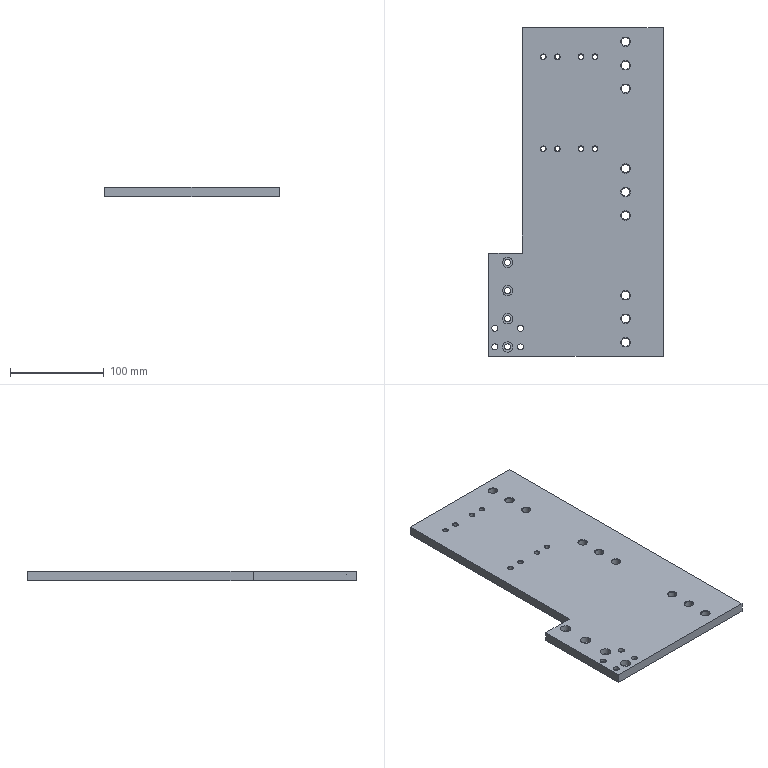Part | NX | features SIMPLE HOLE 25, SYMBOLIC_THREAD 17, DATUM_CSYS 10, HOLE PACKAGE 9, SKETCH 9, EXTRACT_FACE 6, CBORE_HOLE 4, Instance Feature 4, Pattern Feature 2, EXTRUDE 1 | 1 solid | 83 faces | box 185.5 x 350 x 10 mm | volume 550667 mm3 | cone 34 | cylinder 33 | plane 16 | commonest cylinder face diameters 9 x9 5.2 x8 6.5 x8 11 x8